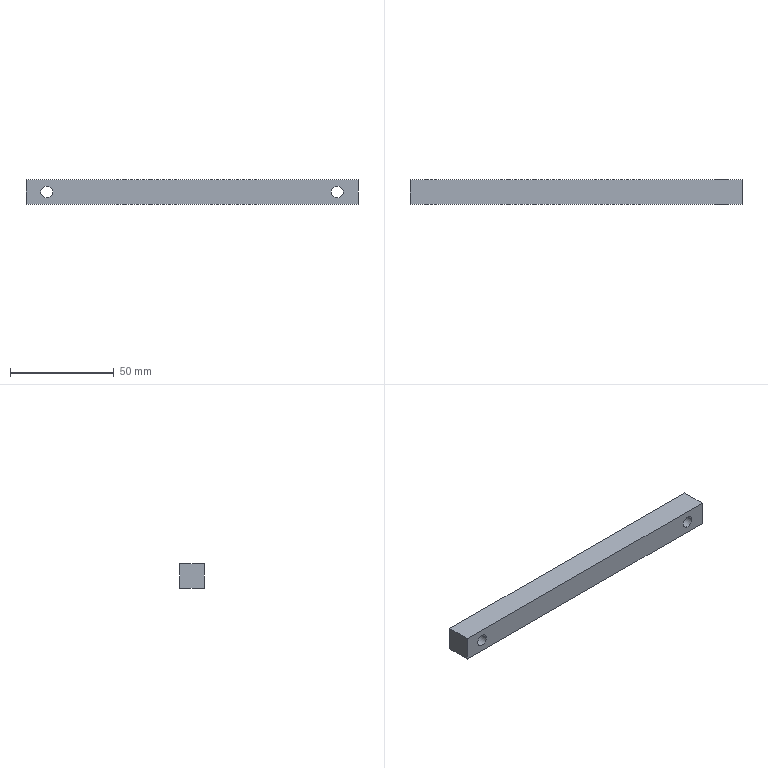Part | STEP file | J013-EBZ05-27-06-Part-1 | 1 solid | 10 faces | box 160 x 12 x 12 mm | volume 22406 mm3 | plane 6 | cylinder 4 | commonest cylinder face diameters 5.8 x4
STEP:
#1=CARTESIAN_POINT('',(147.1,12.,6.));
#2=VERTEX_POINT('',#1);
#3=CARTESIAN_POINT('',(152.9,12.,6.));
#4=VERTEX_POINT('',#3);
#5=CARTESIAN_POINT('',(150.,12.,6.));
#6=DIRECTION('',(0.,-1.,0.));
#7=DIRECTION('',(1.,0.,0.));
#8=AXIS2_PLACEMENT_3D('',#5,#6,#7);
#9=CIRCLE('',#8,2.9);
#10=EDGE_CURVE('',#2,#4,#9,.T.);
#11=ORIENTED_EDGE('',*,*,#10,.F.);
#12=CARTESIAN_POINT('',(147.1,0.,6.));
#13=VERTEX_POINT('',#12);
#14=CARTESIAN_POINT('',(147.1,12.,6.));
#15=DIRECTION('',(0.,-1.,0.));
#16=VECTOR('',#15,1000.);
#17=LINE('',#14,#16);
#18=EDGE_CURVE('',#2,#13,#17,.T.);
#19=ORIENTED_EDGE('',*,*,#18,.T.);
#20=CARTESIAN_POINT('',(152.9,0.,6.));
#21=VERTEX_POINT('',#20);
#22=CARTESIAN_POINT('',(150.,0.,6.));
#23=DIRECTION('',(0.,1.,0.));
#24=DIRECTION('',(-1.,0.,0.));
#25=AXIS2_PLACEMENT_3D('',#22,#23,#24);
#26=CIRCLE('',#25,2.9);
#27=EDGE_CURVE('',#21,#13,#26,.T.);
#28=ORIENTED_EDGE('',*,*,#27,.F.);
#29=CARTESIAN_POINT('',(152.9,12.,6.));
#30=DIRECTION('',(0.,-1.,0.));
#31=VECTOR('',#30,1000.);
#32=LINE('',#29,#31);
#33=EDGE_CURVE('',#4,#21,#32,.T.);
#34=ORIENTED_EDGE('',*,*,#33,.F.);
#35=EDGE_LOOP('',(#11,#19,#28,#34));
#36=FACE_OUTER_BOUND('',#35,.T.);
#37=CARTESIAN_POINT('',(150.,12.,6.));
#38=DIRECTION('',(0.,-1.,0.));
#39=DIRECTION('',(1.,0.,0.));
#40=AXIS2_PLACEMENT_3D('',#37,#38,#39);
#41=CYLINDRICAL_SURFACE('',#40,2.9);
#42=ADVANCED_FACE('',(#36),#41,.F.);
#43=CARTESIAN_POINT('',(7.1,12.,6.));
#44=VERTEX_POINT('',#43);
#45=CARTESIAN_POINT('',(12.9,12.,6.));
#46=VERTEX_POINT('',#45);
#47=CARTESIAN_POINT('',(10.,12.,6.));
#48=DIRECTION('',(0.,-1.,0.));
#49=DIRECTION('',(1.,0.,0.));
#50=AXIS2_PLACEMENT_3D('',#47,#48,#49);
#51=CIRCLE('',#50,2.9);
#52=EDGE_CURVE('',#44,#46,#51,.T.);
#53=ORIENTED_EDGE('',*,*,#52,.F.);
#54=CARTESIAN_POINT('',(7.1,0.,6.));
#55=VERTEX_POINT('',#54);
#56=CARTESIAN_POINT('',(7.1,12.,6.));
#57=DIRECTION('',(0.,-1.,0.));
#58=VECTOR('',#57,1000.);
#59=LINE('',#56,#58);
#60=EDGE_CURVE('',#44,#55,#59,.T.);
#61=ORIENTED_EDGE('',*,*,#60,.T.);
#62=CARTESIAN_POINT('',(12.9,0.,6.));
#63=VERTEX_POINT('',#62);
#64=CARTESIAN_POINT('',(10.,0.,6.));
#65=DIRECTION('',(0.,1.,0.));
#66=DIRECTION('',(-1.,0.,0.));
#67=AXIS2_PLACEMENT_3D('',#64,#65,#66);
#68=CIRCLE('',#67,2.9);
#69=EDGE_CURVE('',#63,#55,#68,.T.);
#70=ORIENTED_EDGE('',*,*,#69,.F.);
#71=CARTESIAN_POINT('',(12.9,12.,6.));
#72=DIRECTION('',(0.,-1.,0.));
#73=VECTOR('',#72,1000.);
#74=LINE('',#71,#73);
#75=EDGE_CURVE('',#46,#63,#74,.T.);
#76=ORIENTED_EDGE('',*,*,#75,.F.);
#77=EDGE_LOOP('',(#53,#61,#70,#76));
#78=FACE_OUTER_BOUND('',#77,.T.);
#79=CARTESIAN_POINT('',(10.,12.,6.));
#80=DIRECTION('',(0.,-1.,0.));
#81=DIRECTION('',(1.,0.,0.));
#82=AXIS2_PLACEMENT_3D('',#79,#80,#81);
#83=CYLINDRICAL_SURFACE('',#82,2.9);
#84=ADVANCED_FACE('',(#78),#83,.F.);
#85=CARTESIAN_POINT('',(0.,0.,12.));
#86=VERTEX_POINT('',#85);
#87=CARTESIAN_POINT('',(0.,0.,0.));
#88=VERTEX_POINT('',#87);
#89=CARTESIAN_POINT('',(0.,0.,6.));
#90=DIRECTION('',(0.,0.,-1.));
#91=VECTOR('',#90,1000.);
#92=LINE('',#89,#91);
#93=EDGE_CURVE('',#86,#88,#92,.T.);
#94=ORIENTED_EDGE('',*,*,#93,.F.);
#95=CARTESIAN_POINT('',(0.,12.,12.));
#96=VERTEX_POINT('',#95);
#97=CARTESIAN_POINT('',(0.,6.,12.));
#98=DIRECTION('',(0.,-1.,0.));
#99=VECTOR('',#98,1000.);
#100=LINE('',#97,#99);
#101=EDGE_CURVE('',#96,#86,#100,.T.);
#102=ORIENTED_EDGE('',*,*,#101,.F.);
#103=CARTESIAN_POINT('',(0.,12.,0.));
#104=VERTEX_POINT('',#103);
#105=CARTESIAN_POINT('',(0.,12.,6.));
#106=DIRECTION('',(0.,0.,1.));
#107=VECTOR('',#106,1000.);
#108=LINE('',#105,#107);
#109=EDGE_CURVE('',#104,#96,#108,.T.);
#110=ORIENTED_EDGE('',*,*,#109,.F.);
#111=CARTESIAN_POINT('',(0.,6.,0.));
#112=DIRECTION('',(0.,1.,0.));
#113=VECTOR('',#112,1000.);
#114=LINE('',#111,#113);
#115=EDGE_CURVE('',#88,#104,#114,.T.);
#116=ORIENTED_EDGE('',*,*,#115,.F.);
#117=EDGE_LOOP('',(#94,#102,#110,#116));
#118=FACE_OUTER_BOUND('',#117,.T.);
#119=CARTESIAN_POINT('',(0.,6.,6.));
#120=DIRECTION('',(-1.,0.,0.));
#121=DIRECTION('',(0.,0.,1.));
#122=AXIS2_PLACEMENT_3D('',#119,#120,#121);
#123=PLANE('',#122);
#124=ADVANCED_FACE('',(#118),#123,.T.);
#125=ORIENTED_EDGE('',*,*,#27,.T.);
#126=CARTESIAN_POINT('',(150.,0.,6.));
#127=DIRECTION('',(0.,1.,0.));
#128=DIRECTION('',(-1.,0.,0.));
#129=AXIS2_PLACEMENT_3D('',#126,#127,#128);
#130=CIRCLE('',#129,2.9);
#131=EDGE_CURVE('',#13,#21,#130,.T.);
#132=ORIENTED_EDGE('',*,*,#131,.T.);
#133=EDGE_LOOP('',(#125,#132));
#134=FACE_BOUND('',#133,.T.);
#135=ORIENTED_EDGE('',*,*,#69,.T.);
#136=CARTESIAN_POINT('',(10.,0.,6.));
#137=DIRECTION('',(0.,1.,0.));
#138=DIRECTION('',(-1.,0.,0.));
#139=AXIS2_PLACEMENT_3D('',#136,#137,#138);
#140=CIRCLE('',#139,2.9);
#141=EDGE_CURVE('',#55,#63,#140,.T.);
#142=ORIENTED_EDGE('',*,*,#141,.T.);
#143=EDGE_LOOP('',(#135,#142));
#144=FACE_BOUND('',#143,.T.);
#145=CARTESIAN_POINT('',(160.,0.,12.));
#146=VERTEX_POINT('',#145);
#147=CARTESIAN_POINT('',(160.,0.,12.));
#148=DIRECTION('',(-1.,0.,0.));
#149=VECTOR('',#148,1000.);
#150=LINE('',#147,#149);
#151=EDGE_CURVE('',#146,#86,#150,.T.);
#152=ORIENTED_EDGE('',*,*,#151,.T.);
#153=ORIENTED_EDGE('',*,*,#93,.T.);
#154=CARTESIAN_POINT('',(160.,0.,0.));
#155=VERTEX_POINT('',#154);
#156=CARTESIAN_POINT('',(160.,0.,0.));
#157=DIRECTION('',(-1.,0.,0.));
#158=VECTOR('',#157,1000.);
#159=LINE('',#156,#158);
#160=EDGE_CURVE('',#155,#88,#159,.T.);
#161=ORIENTED_EDGE('',*,*,#160,.F.);
#162=CARTESIAN_POINT('',(160.,0.,6.));
#163=DIRECTION('',(0.,0.,1.));
#164=VECTOR('',#163,1000.);
#165=LINE('',#162,#164);
#166=EDGE_CURVE('',#155,#146,#165,.T.);
#167=ORIENTED_EDGE('',*,*,#166,.T.);
#168=EDGE_LOOP('',(#152,#153,#161,#167));
#169=FACE_OUTER_BOUND('',#168,.T.);
#170=CARTESIAN_POINT('',(160.,0.,6.));
#171=DIRECTION('',(0.,-1.,0.));
#172=DIRECTION('',(1.,0.,0.));
#173=AXIS2_PLACEMENT_3D('',#170,#171,#172);
#174=PLANE('',#173);
#175=ADVANCED_FACE('',(#134,#144,#169),#174,.T.);
#176=ORIENTED_EDGE('',*,*,#160,.T.);
#177=ORIENTED_EDGE('',*,*,#115,.T.);
#178=CARTESIAN_POINT('',(160.,12.,0.));
#179=VERTEX_POINT('',#178);
#180=CARTESIAN_POINT('',(160.,12.,0.));
#181=DIRECTION('',(-1.,0.,0.));
#182=VECTOR('',#181,1000.);
#183=LINE('',#180,#182);
#184=EDGE_CURVE('',#179,#104,#183,.T.);
#185=ORIENTED_EDGE('',*,*,#184,.F.);
#186=CARTESIAN_POINT('',(160.,6.,0.));
#187=DIRECTION('',(0.,-1.,0.));
#188=VECTOR('',#187,1000.);
#189=LINE('',#186,#188);
#190=EDGE_CURVE('',#179,#155,#189,.T.);
#191=ORIENTED_EDGE('',*,*,#190,.T.);
#192=EDGE_LOOP('',(#176,#177,#185,#191));
#193=FACE_OUTER_BOUND('',#192,.T.);
#194=CARTESIAN_POINT('',(160.,6.,0.));
#195=DIRECTION('',(0.,0.,-1.));
#196=DIRECTION('',(-1.,0.,0.));
#197=AXIS2_PLACEMENT_3D('',#194,#195,#196);
#198=PLANE('',#197);
#199=ADVANCED_FACE('',(#193),#198,.T.);
#200=CARTESIAN_POINT('',(150.,12.,6.));
#201=DIRECTION('',(0.,-1.,0.));
#202=DIRECTION('',(1.,0.,0.));
#203=AXIS2_PLACEMENT_3D('',#200,#201,#202);
#204=CIRCLE('',#203,2.9);
#205=EDGE_CURVE('',#4,#2,#204,.T.);
#206=ORIENTED_EDGE('',*,*,#205,.T.);
#207=ORIENTED_EDGE('',*,*,#10,.T.);
#208=EDGE_LOOP('',(#206,#207));
#209=FACE_BOUND('',#208,.T.);
#210=CARTESIAN_POINT('',(10.,12.,6.));
#211=DIRECTION('',(0.,-1.,0.));
#212=DIRECTION('',(1.,0.,0.));
#213=AXIS2_PLACEMENT_3D('',#210,#211,#212);
#214=CIRCLE('',#213,2.9);
#215=EDGE_CURVE('',#46,#44,#214,.T.);
#216=ORIENTED_EDGE('',*,*,#215,.T.);
#217=ORIENTED_EDGE('',*,*,#52,.T.);
#218=EDGE_LOOP('',(#216,#217));
#219=FACE_BOUND('',#218,.T.);
#220=ORIENTED_EDGE('',*,*,#184,.T.);
#221=ORIENTED_EDGE('',*,*,#109,.T.);
#222=CARTESIAN_POINT('',(160.,12.,12.));
#223=VERTEX_POINT('',#222);
#224=CARTESIAN_POINT('',(160.,12.,12.));
#225=DIRECTION('',(-1.,0.,0.));
#226=VECTOR('',#225,1000.);
#227=LINE('',#224,#226);
#228=EDGE_CURVE('',#223,#96,#227,.T.);
#229=ORIENTED_EDGE('',*,*,#228,.F.);
#230=CARTESIAN_POINT('',(160.,12.,6.));
#231=DIRECTION('',(0.,0.,-1.));
#232=VECTOR('',#231,1000.);
#233=LINE('',#230,#232);
#234=EDGE_CURVE('',#223,#179,#233,.T.);
#235=ORIENTED_EDGE('',*,*,#234,.T.);
#236=EDGE_LOOP('',(#220,#221,#229,#235));
#237=FACE_OUTER_BOUND('',#236,.T.);
#238=CARTESIAN_POINT('',(160.,12.,6.));
#239=DIRECTION('',(0.,1.,0.));
#240=DIRECTION('',(-1.,0.,0.));
#241=AXIS2_PLACEMENT_3D('',#238,#239,#240);
#242=PLANE('',#241);
#243=ADVANCED_FACE('',(#209,#219,#237),#242,.T.);
#244=CARTESIAN_POINT('',(160.,6.,12.));
#245=DIRECTION('',(0.,1.,0.));
#246=VECTOR('',#245,1000.);
#247=LINE('',#244,#246);
#248=EDGE_CURVE('',#146,#223,#247,.T.);
#249=ORIENTED_EDGE('',*,*,#248,.F.);
#250=ORIENTED_EDGE('',*,*,#166,.F.);
#251=ORIENTED_EDGE('',*,*,#190,.F.);
#252=ORIENTED_EDGE('',*,*,#234,.F.);
#253=EDGE_LOOP('',(#249,#250,#251,#252));
#254=FACE_OUTER_BOUND('',#253,.T.);
#255=CARTESIAN_POINT('',(160.,6.,6.));
#256=DIRECTION('',(1.,0.,0.));
#257=DIRECTION('',(0.,0.,-1.));
#258=AXIS2_PLACEMENT_3D('',#255,#256,#257);
#259=PLANE('',#258);
#260=ADVANCED_FACE('',(#254),#259,.T.);
#261=ORIENTED_EDGE('',*,*,#248,.T.);
#262=ORIENTED_EDGE('',*,*,#228,.T.);
#263=ORIENTED_EDGE('',*,*,#101,.T.);
#264=ORIENTED_EDGE('',*,*,#151,.F.);
#265=EDGE_LOOP('',(#261,#262,#263,#264));
#266=FACE_OUTER_BOUND('',#265,.T.);
#267=CARTESIAN_POINT('',(160.,6.,12.));
#268=DIRECTION('',(0.,0.,1.));
#269=DIRECTION('',(1.,0.,0.));
#270=AXIS2_PLACEMENT_3D('',#267,#268,#269);
#271=PLANE('',#270);
#272=ADVANCED_FACE('',(#266),#271,.T.);
#273=ORIENTED_EDGE('',*,*,#60,.F.);
#274=ORIENTED_EDGE('',*,*,#215,.F.);
#275=ORIENTED_EDGE('',*,*,#75,.T.);
#276=ORIENTED_EDGE('',*,*,#141,.F.);
#277=EDGE_LOOP('',(#273,#274,#275,#276));
#278=FACE_OUTER_BOUND('',#277,.T.);
#279=CARTESIAN_POINT('',(10.,12.,6.));
#280=DIRECTION('',(0.,-1.,0.));
#281=DIRECTION('',(1.,0.,0.));
#282=AXIS2_PLACEMENT_3D('',#279,#280,#281);
#283=CYLINDRICAL_SURFACE('',#282,2.9);
#284=ADVANCED_FACE('',(#278),#283,.F.);
#285=ORIENTED_EDGE('',*,*,#18,.F.);
#286=ORIENTED_EDGE('',*,*,#205,.F.);
#287=ORIENTED_EDGE('',*,*,#33,.T.);
#288=ORIENTED_EDGE('',*,*,#131,.F.);
#289=EDGE_LOOP('',(#285,#286,#287,#288));
#290=FACE_OUTER_BOUND('',#289,.T.);
#291=CARTESIAN_POINT('',(150.,12.,6.));
#292=DIRECTION('',(0.,-1.,0.));
#293=DIRECTION('',(1.,0.,0.));
#294=AXIS2_PLACEMENT_3D('',#291,#292,#293);
#295=CYLINDRICAL_SURFACE('',#294,2.9);
#296=ADVANCED_FACE('',(#290),#295,.F.);
#297=CLOSED_SHELL('',(#42,#84,#124,#175,#199,#243,#260,#272,#284,#296));
#298=MANIFOLD_SOLID_BREP('',#297);
#299=CARTESIAN_POINT('',(0.,0.,0.));
#300=DIRECTION('',(0.,0.,1.));
#301=DIRECTION('',(1.,0.,0.));
#302=AXIS2_PLACEMENT_3D('',#299,#300,#301);
#303=(LENGTH_UNIT()NAMED_UNIT(*)SI_UNIT(.MILLI.,.METRE.));
#304=UNCERTAINTY_MEASURE_WITH_UNIT(LENGTH_MEASURE(0.00001),#303,'','');
#305=(NAMED_UNIT(*)PLANE_ANGLE_UNIT()SI_UNIT($,.RADIAN.));
#306=(NAMED_UNIT(*)SI_UNIT($,.STERADIAN.)SOLID_ANGLE_UNIT());
#307=(GEOMETRIC_REPRESENTATION_CONTEXT(3)GLOBAL_UNCERTAINTY_ASSIGNED_CONTEXT((#304))GLOBAL_UNIT_ASSIGNED_CONTEXT((#303,#305,#306))REPRESENTATION_CONTEXT('',''));
#308=ADVANCED_BREP_SHAPE_REPRESENTATION('',(#298,#302),#307);